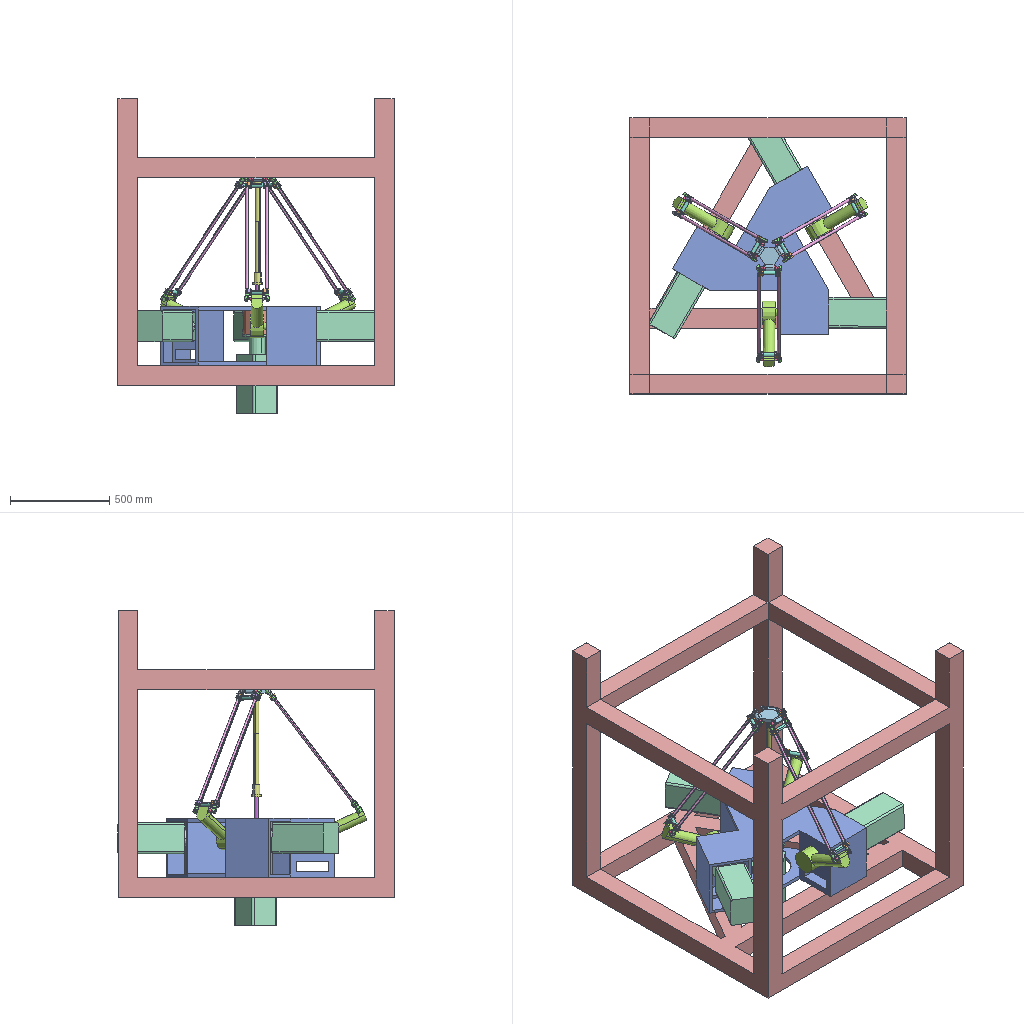Assembly | SolidWorks | 13 different items | 46 placed | box 1395 x 1396 x 1590 mm
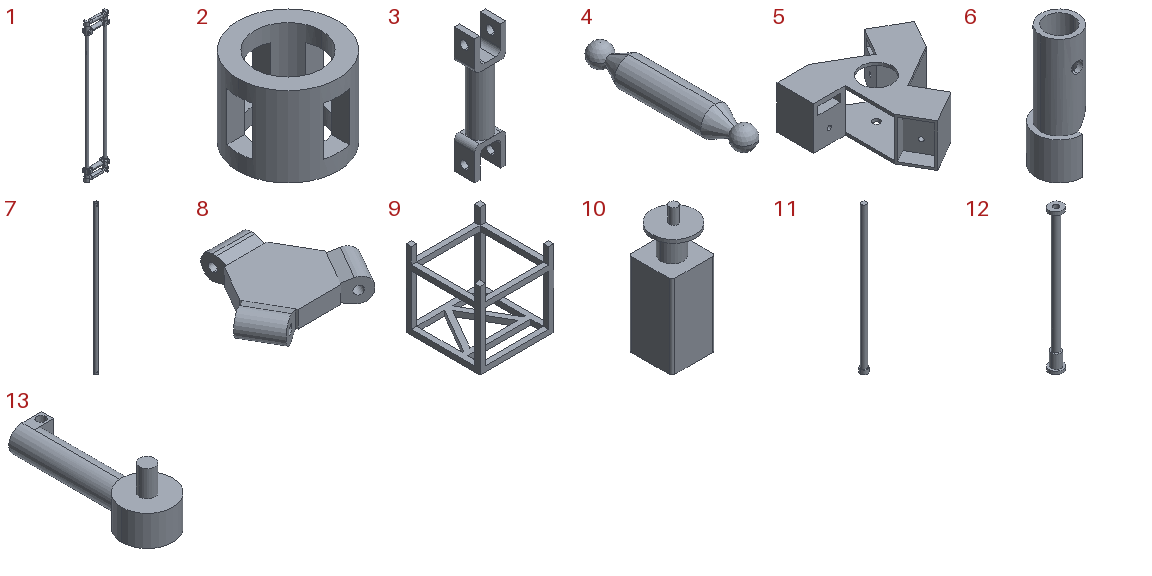Parts list (item | name | quantity | parent item | size | volume | features):
1 | (subassembly) | x3 | - | 125 x 30 x 780 mm | 248012 mm3 | features CompositeCurve 2
2 | - | x1 | - | 150 x 150 x 120 mm | 893145 mm3 | features CirPattern 1, Extrusion 1, ICE 1
3 | - | x6 | in 1 | 30 x 20 x 120 mm | 33900 mm3 | features ICE 2, Extrusion 1
4 | - | x6 | in 1 | 20 x 115 x 20 mm | 26386 mm3 | features Revolution 1
5 | - | x1 | - | 849.615 x 808.551 x 300 mm | 36115158 mm3 | features ICE 7, CirPattern 1, Extrusion 1
6 | - | x12 | in 1 | 22.5 x 25 x 65 mm | 9681 mm3 | features ICE 3, Extrusion 1, RevCut 1
7 | - | x6 | in 1 | 15 x 15 x 700 mm | 44358 mm3 | features Extrusion 1, ICE 1
8 | - | x1 | - | 149.462 x 129.437 x 28 mm | 213673 mm3 | features ICE 2, CirPattern 1, Extrusion 1
9 | - | x1 | - | 1395 x 1395 x 1450 mm | 185057639 mm3 | features ICE 3, Extrusion 1
10 | - | x4 | - | 161.788 x 156 x 455 mm | 7985623 mm3 | features ICE 3, Extrusion 1, Fillet 1
11 | - | x1 | - | 25 x 25 x 515 mm | 134598 mm3 | features Extrusion 1, ICE 1
12 | - | x1 | - | 50 x 50 x 524 mm | 151503 mm3 | features ICE 4, Extrusion 1
13 | - | x3 | - | 117 x 346.5 x 130 mm | 1482010 mm3 | features ICE 4, Extrusion 1
Mates (type | each side: item.copy, entity, surface, feature):
In the top assembly
Concentric | 13.1 face cylinder Cut-Extrude1 | 4.1 face cylinder Revolve1
DistanceDim | 6.1 face plane Cut-Extrude2 | 13.1 face plane Boss-Extrude4
Concentric | 4.2 face cylinder Revolve1 | 8.1 face cylinder Boss-Extrude2
Coincident | 9.1 face plane Boss-Extrude1 | 5.1 face plane Boss-Extrude1
Parallel | 9.1 face plane Boss-Extrude1 | 5.1 face plane Boss-Extrude1
Concentric | 5.1 face cylinder Cut-Extrude6 | 13.1 face cylinder Boss-Extrude6
Concentric | 5.1 face cylinder Cut-Extrude3 | 8.1 face cylinder Cut-Extrude1
DistanceDim | 8.1 face plane Boss-Extrude2 | 7.1 face cylinder Boss-Extrude1
Concentric | 8.1 face cylinder Cut-Extrude1 | 12.1 face cylinder Boss-Extrude4
Coincident | 8.1 face plane Boss-Extrude1 | 12.1 face plane Boss-Extrude4
Concentric | 12.1 face cylinder Boss-Extrude1 | 11.1 face cylinder Boss-Extrude1
Concentric | 5.1 face cylinder Cut-Extrude6 | 10.1 face cylinder Boss-Extrude2
Coincident | 5.1 face plane CirPattern1 | 10.1 face plane Boss-Extrude3
Coincident | 5.1 face plane Cut-Extrude2 | 2.1 face plane Boss-Extrude1
Concentric | 5.1 face cylinder Cut-Extrude3 | 2.1 face cylinder Boss-Extrude1
Coincident | 2.1 face plane Boss-Extrude1 | 10.2 face plane Boss-Extrude3
Coincident | 11.1 face plane Boss-Extrude2 | 10.2 face plane Boss-Extrude4
Concentric | 2.1 face cylinder Boss-Extrude1 | 10.2 face cylinder Boss-Extrude3
In subassembly 1
Concentric | 7.2 face cylinder Cut-Extrude1 | 3.1 face cylinder Cut-Extrude1
DistanceDim | 7.2 face cylinder Boss-Extrude1 | 3.1 face plane Boss-Extrude2
Concentric | 3.1 face cylinder Cut-Extrude1 | 7.3 face cylinder Cut-Extrude1
DistanceDim | 7.3 face cylinder Boss-Extrude1 | 3.1 face plane Boss-Extrude2
Concentric | 7.3 face cylinder Cut-Extrude1 | 3.2 face cylinder Cut-Extrude1
Concentric | 7.2 face cylinder Cut-Extrude1 | 3.2 face cylinder Cut-Extrude1
Coincident | 3.1 face plane Boss-Extrude2 | 3.2 face plane Boss-Extrude2
Coincident | 7.2 face plane Boss-Extrude1 | 7.3 face plane Boss-Extrude1
Concentric | 7.2 face cylinder Boss-Extrude1 | 6.2 face cylinder Boss-Extrude1
Concentric | 3.2 face cylinder Cut-Extrude1 | 6.2 face cylinder Cut-Extrude1
Concentric | 7.3 face cylinder Boss-Extrude1 | 6.3 face cylinder Boss-Extrude1
Concentric | 3.2 face cylinder Cut-Extrude1 | 6.3 face cylinder Cut-Extrude1
Concentric | 7.3 face cylinder Boss-Extrude1 | 6.4 face cylinder Boss-Extrude1
Concentric | 3.1 face cylinder Cut-Extrude1 | 6.4 face cylinder Cut-Extrude1
Concentric | 7.2 face cylinder Boss-Extrude1 | 6.5 face cylinder Boss-Extrude1
Concentric | 3.1 face cylinder Cut-Extrude1 | 6.5 face cylinder Cut-Extrude1
Concentric | 6.5 face sphere Cut-Revolve3 | 4.3 face sphere Revolve1
Tangent | 6.4 edge | 4.3 face sphere Revolve1
Concentric | 6.3 face sphere Cut-Revolve3 | 4.4 face sphere Revolve1
Tangent | 6.2 edge | 4.4 face sphere Revolve1